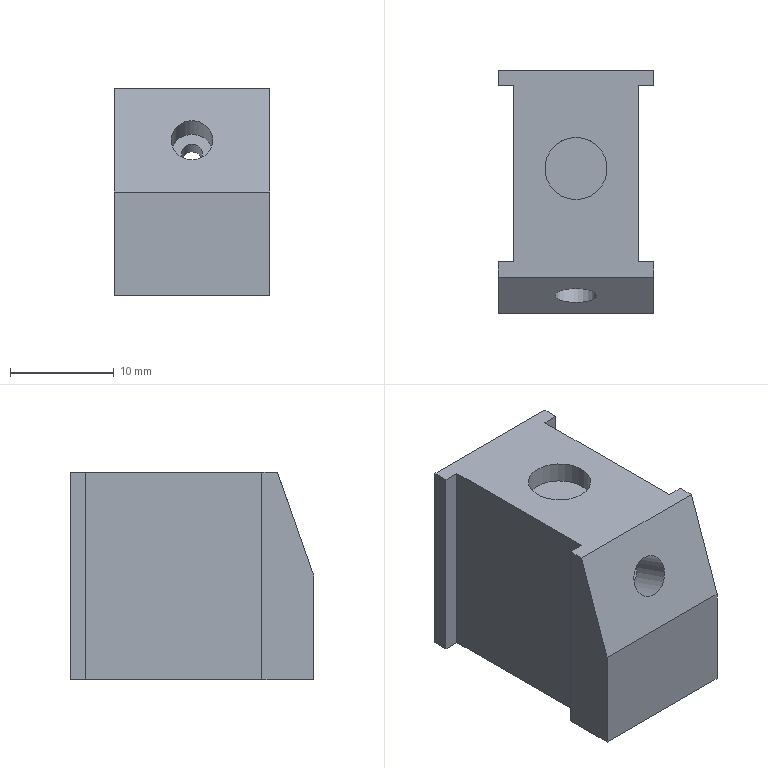Part | STEP file | 1-41.3 | 1 solid | 22 faces | box 15 x 23.5 x 20 mm | volume 4873 mm3 | plane 18 | cylinder 4 | commonest cylinder face diameters 2 x1 4 x1 6 x1 8 x1